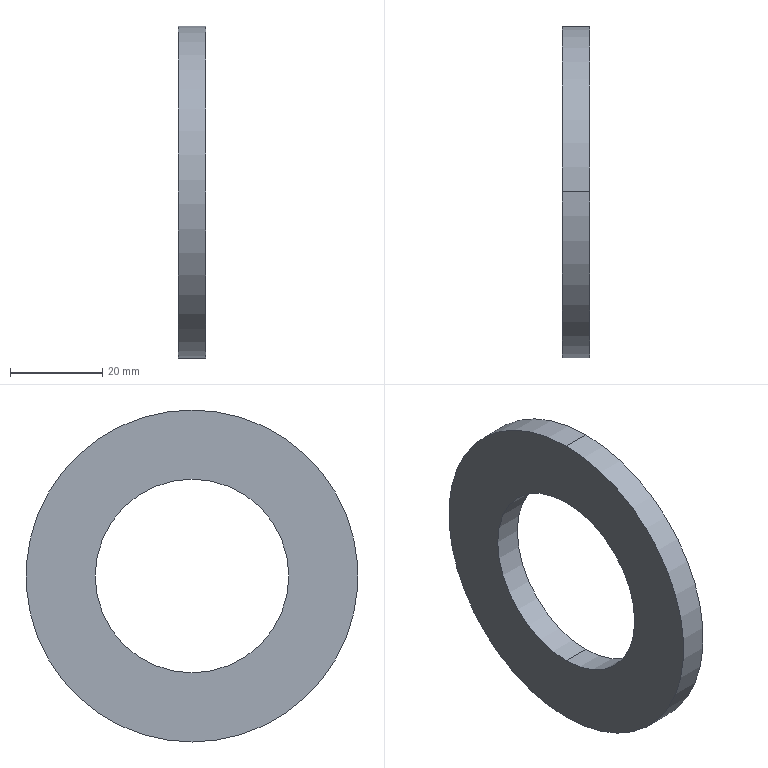Part | STEP file | 1 solid | 6 faces | box 6 x 72 x 72 mm | volume 16116 mm3 | cylinder 4 | plane 2 | commonest cylinder face diameters 42 x2 72 x2
STEP:
#1=CARTESIAN_POINT('',(0.,0.,0.));
#2=DIRECTION('',(0.,0.,1.));
#3=DIRECTION('',(1.,0.,0.));
#4=AXIS2_PLACEMENT_3D('',#1,#2,#3);
#5=CARTESIAN_POINT('',(0.,0.,36.));
#6=VERTEX_POINT('',#5);
#7=CARTESIAN_POINT('',(0.,0.,-36.));
#8=VERTEX_POINT('',#7);
#9=CARTESIAN_POINT('',(0.,0.,0.));
#10=DIRECTION('',(-1.,0.,0.));
#11=DIRECTION('',(0.,0.,-1.));
#12=AXIS2_PLACEMENT_3D('',#9,#10,#11);
#13=CIRCLE('',#12,36.);
#14=CARTESIAN_POINT('',(0.,0.,0.));
#15=DIRECTION('',(1.,0.,0.));
#16=DIRECTION('',(0.,0.,-1.));
#17=AXIS2_PLACEMENT_3D('',#14,#15,#16);
#18=CYLINDRICAL_SURFACE('',#17,36.);
#19=CARTESIAN_POINT('',(6.283,0.));
#20=DIRECTION('',(-1.,0.));
#21=VECTOR('',#20,1.);
#22=LINE('',#19,#21);
#23=(GEOMETRIC_REPRESENTATION_CONTEXT(2)PARAMETRIC_REPRESENTATION_CONTEXT()REPRESENTATION_CONTEXT('',''));
#24=DEFINITIONAL_REPRESENTATION('',(#22),#23);
#25=PCURVE('',#18,#24);
#26=CARTESIAN_POINT('',(0.,0.,0.));
#27=DIRECTION('',(-1.,0.,0.));
#28=DIRECTION('',(0.,0.,1.));
#29=AXIS2_PLACEMENT_3D('',#26,#27,#28);
#30=PLANE('',#29);
#31=CARTESIAN_POINT('',(0.,0.));
#32=DIRECTION('',(-1.,0.));
#33=AXIS2_PLACEMENT_2D('',#31,#32);
#34=CIRCLE('',#33,36.);
#35=(GEOMETRIC_REPRESENTATION_CONTEXT(2)PARAMETRIC_REPRESENTATION_CONTEXT()REPRESENTATION_CONTEXT('',''));
#36=DEFINITIONAL_REPRESENTATION('',(#34),#35);
#37=PCURVE('',#30,#36);
#38=SURFACE_CURVE('',#13,(#25,#37),.PCURVE_S1.);
#39=EDGE_CURVE('',#6,#8,#38,.T.);
#40=ORIENTED_EDGE('',*,*,#39,.F.);
#41=CARTESIAN_POINT('',(6.,0.,36.));
#42=VERTEX_POINT('',#41);
#43=CARTESIAN_POINT('',(0.,0.,36.));
#44=DIRECTION('',(1.,0.,0.));
#45=VECTOR('',#44,1.);
#46=LINE('',#43,#45);
#47=CARTESIAN_POINT('',(3.142,0.));
#48=DIRECTION('',(0.,1.));
#49=VECTOR('',#48,1.);
#50=LINE('',#47,#49);
#51=(GEOMETRIC_REPRESENTATION_CONTEXT(2)PARAMETRIC_REPRESENTATION_CONTEXT()REPRESENTATION_CONTEXT('',''));
#52=DEFINITIONAL_REPRESENTATION('',(#50),#51);
#53=PCURVE('',#18,#52);
#54=CARTESIAN_POINT('',(0.,0.,0.));
#55=DIRECTION('',(1.,0.,0.));
#56=DIRECTION('',(0.,0.,-1.));
#57=AXIS2_PLACEMENT_3D('',#54,#55,#56);
#58=CYLINDRICAL_SURFACE('',#57,36.);
#59=CARTESIAN_POINT('',(3.142,0.));
#60=DIRECTION('',(0.,1.));
#61=VECTOR('',#60,1.);
#62=LINE('',#59,#61);
#63=(GEOMETRIC_REPRESENTATION_CONTEXT(2)PARAMETRIC_REPRESENTATION_CONTEXT()REPRESENTATION_CONTEXT('',''));
#64=DEFINITIONAL_REPRESENTATION('',(#62),#63);
#65=PCURVE('',#58,#64);
#66=SURFACE_CURVE('',#46,(#53,#65),.PCURVE_S1.);
#67=EDGE_CURVE('',#6,#42,#66,.T.);
#68=ORIENTED_EDGE('',*,*,#67,.T.);
#69=CARTESIAN_POINT('',(6.,0.,-36.));
#70=VERTEX_POINT('',#69);
#71=CARTESIAN_POINT('',(6.,0.,0.));
#72=DIRECTION('',(-1.,0.,0.));
#73=DIRECTION('',(0.,0.,-1.));
#74=AXIS2_PLACEMENT_3D('',#71,#72,#73);
#75=CIRCLE('',#74,36.);
#76=CARTESIAN_POINT('',(6.283,6.));
#77=DIRECTION('',(-1.,0.));
#78=VECTOR('',#77,1.);
#79=LINE('',#76,#78);
#80=(GEOMETRIC_REPRESENTATION_CONTEXT(2)PARAMETRIC_REPRESENTATION_CONTEXT()REPRESENTATION_CONTEXT('',''));
#81=DEFINITIONAL_REPRESENTATION('',(#79),#80);
#82=PCURVE('',#18,#81);
#83=CARTESIAN_POINT('',(6.,0.,0.));
#84=DIRECTION('',(-1.,0.,0.));
#85=DIRECTION('',(0.,0.,1.));
#86=AXIS2_PLACEMENT_3D('',#83,#84,#85);
#87=PLANE('',#86);
#88=CARTESIAN_POINT('',(0.,0.));
#89=DIRECTION('',(-1.,0.));
#90=AXIS2_PLACEMENT_2D('',#88,#89);
#91=CIRCLE('',#90,36.);
#92=(GEOMETRIC_REPRESENTATION_CONTEXT(2)PARAMETRIC_REPRESENTATION_CONTEXT()REPRESENTATION_CONTEXT('',''));
#93=DEFINITIONAL_REPRESENTATION('',(#91),#92);
#94=PCURVE('',#87,#93);
#95=SURFACE_CURVE('',#75,(#82,#94),.PCURVE_S1.);
#96=EDGE_CURVE('',#42,#70,#95,.T.);
#97=ORIENTED_EDGE('',*,*,#96,.T.);
#98=CARTESIAN_POINT('',(0.,0.,-36.));
#99=DIRECTION('',(1.,0.,0.));
#100=VECTOR('',#99,1.);
#101=LINE('',#98,#100);
#102=CARTESIAN_POINT('',(0.,0.));
#103=DIRECTION('',(0.,1.));
#104=VECTOR('',#103,1.);
#105=LINE('',#102,#104);
#106=(GEOMETRIC_REPRESENTATION_CONTEXT(2)PARAMETRIC_REPRESENTATION_CONTEXT()REPRESENTATION_CONTEXT('',''));
#107=DEFINITIONAL_REPRESENTATION('',(#105),#106);
#108=PCURVE('',#18,#107);
#109=CARTESIAN_POINT('',(6.283,0.));
#110=DIRECTION('',(0.,1.));
#111=VECTOR('',#110,1.);
#112=LINE('',#109,#111);
#113=(GEOMETRIC_REPRESENTATION_CONTEXT(2)PARAMETRIC_REPRESENTATION_CONTEXT()REPRESENTATION_CONTEXT('',''));
#114=DEFINITIONAL_REPRESENTATION('',(#112),#113);
#115=PCURVE('',#58,#114);
#116=SURFACE_CURVE('',#101,(#108,#115),.PCURVE_S1.);
#117=EDGE_CURVE('',#8,#70,#116,.T.);
#118=ORIENTED_EDGE('',*,*,#117,.F.);
#119=EDGE_LOOP('',(#40,#68,#97,#118));
#120=FACE_BOUND('',#119,.T.);
#121=ADVANCED_FACE('',(#120),#18,.T.);
#122=CARTESIAN_POINT('',(0.,0.,-21.));
#123=VERTEX_POINT('',#122);
#124=CARTESIAN_POINT('',(6.,0.,-21.));
#125=VERTEX_POINT('',#124);
#126=CARTESIAN_POINT('',(0.,0.,-21.));
#127=DIRECTION('',(1.,0.,0.));
#128=VECTOR('',#127,1.);
#129=LINE('',#126,#128);
#130=CARTESIAN_POINT('',(0.,0.,0.));
#131=DIRECTION('',(1.,0.,0.));
#132=DIRECTION('',(0.,0.,-1.));
#133=AXIS2_PLACEMENT_3D('',#130,#131,#132);
#134=CYLINDRICAL_SURFACE('',#133,21.);
#135=CARTESIAN_POINT('',(6.283,0.));
#136=DIRECTION('',(0.,1.));
#137=VECTOR('',#136,1.);
#138=LINE('',#135,#137);
#139=(GEOMETRIC_REPRESENTATION_CONTEXT(2)PARAMETRIC_REPRESENTATION_CONTEXT()REPRESENTATION_CONTEXT('',''));
#140=DEFINITIONAL_REPRESENTATION('',(#138),#139);
#141=PCURVE('',#134,#140);
#142=CARTESIAN_POINT('',(0.,0.,0.));
#143=DIRECTION('',(1.,0.,0.));
#144=DIRECTION('',(0.,0.,-1.));
#145=AXIS2_PLACEMENT_3D('',#142,#143,#144);
#146=CYLINDRICAL_SURFACE('',#145,21.);
#147=CARTESIAN_POINT('',(0.,0.));
#148=DIRECTION('',(0.,1.));
#149=VECTOR('',#148,1.);
#150=LINE('',#147,#149);
#151=(GEOMETRIC_REPRESENTATION_CONTEXT(2)PARAMETRIC_REPRESENTATION_CONTEXT()REPRESENTATION_CONTEXT('',''));
#152=DEFINITIONAL_REPRESENTATION('',(#150),#151);
#153=PCURVE('',#146,#152);
#154=SURFACE_CURVE('',#129,(#141,#153),.PCURVE_S1.);
#155=EDGE_CURVE('',#123,#125,#154,.T.);
#156=ORIENTED_EDGE('',*,*,#155,.T.);
#157=CARTESIAN_POINT('',(6.,0.,21.));
#158=VERTEX_POINT('',#157);
#159=CARTESIAN_POINT('',(6.,0.,0.));
#160=DIRECTION('',(-1.,0.,0.));
#161=DIRECTION('',(0.,0.,-1.));
#162=AXIS2_PLACEMENT_3D('',#159,#160,#161);
#163=CIRCLE('',#162,21.);
#164=CARTESIAN_POINT('',(6.283,6.));
#165=DIRECTION('',(-1.,0.));
#166=VECTOR('',#165,1.);
#167=LINE('',#164,#166);
#168=(GEOMETRIC_REPRESENTATION_CONTEXT(2)PARAMETRIC_REPRESENTATION_CONTEXT()REPRESENTATION_CONTEXT('',''));
#169=DEFINITIONAL_REPRESENTATION('',(#167),#168);
#170=PCURVE('',#134,#169);
#171=CARTESIAN_POINT('',(0.,0.));
#172=DIRECTION('',(-1.,0.));
#173=AXIS2_PLACEMENT_2D('',#171,#172);
#174=CIRCLE('',#173,21.);
#175=(GEOMETRIC_REPRESENTATION_CONTEXT(2)PARAMETRIC_REPRESENTATION_CONTEXT()REPRESENTATION_CONTEXT('',''));
#176=DEFINITIONAL_REPRESENTATION('',(#174),#175);
#177=PCURVE('',#87,#176);
#178=SURFACE_CURVE('',#163,(#170,#177),.PCURVE_S1.);
#179=EDGE_CURVE('',#125,#158,#178,.T.);
#180=ORIENTED_EDGE('',*,*,#179,.T.);
#181=CARTESIAN_POINT('',(0.,0.,21.));
#182=VERTEX_POINT('',#181);
#183=CARTESIAN_POINT('',(0.,0.,21.));
#184=DIRECTION('',(1.,0.,0.));
#185=VECTOR('',#184,1.);
#186=LINE('',#183,#185);
#187=CARTESIAN_POINT('',(3.142,0.));
#188=DIRECTION('',(0.,1.));
#189=VECTOR('',#188,1.);
#190=LINE('',#187,#189);
#191=(GEOMETRIC_REPRESENTATION_CONTEXT(2)PARAMETRIC_REPRESENTATION_CONTEXT()REPRESENTATION_CONTEXT('',''));
#192=DEFINITIONAL_REPRESENTATION('',(#190),#191);
#193=PCURVE('',#134,#192);
#194=CARTESIAN_POINT('',(3.142,0.));
#195=DIRECTION('',(0.,1.));
#196=VECTOR('',#195,1.);
#197=LINE('',#194,#196);
#198=(GEOMETRIC_REPRESENTATION_CONTEXT(2)PARAMETRIC_REPRESENTATION_CONTEXT()REPRESENTATION_CONTEXT('',''));
#199=DEFINITIONAL_REPRESENTATION('',(#197),#198);
#200=PCURVE('',#146,#199);
#201=SURFACE_CURVE('',#186,(#193,#200),.PCURVE_S1.);
#202=EDGE_CURVE('',#182,#158,#201,.T.);
#203=ORIENTED_EDGE('',*,*,#202,.F.);
#204=CARTESIAN_POINT('',(0.,0.,0.));
#205=DIRECTION('',(1.,0.,0.));
#206=DIRECTION('',(0.,0.,-1.));
#207=AXIS2_PLACEMENT_3D('',#204,#205,#206);
#208=CIRCLE('',#207,21.);
#209=CARTESIAN_POINT('',(0.,0.));
#210=DIRECTION('',(1.,0.));
#211=VECTOR('',#210,1.);
#212=LINE('',#209,#211);
#213=(GEOMETRIC_REPRESENTATION_CONTEXT(2)PARAMETRIC_REPRESENTATION_CONTEXT()REPRESENTATION_CONTEXT('',''));
#214=DEFINITIONAL_REPRESENTATION('',(#212),#213);
#215=PCURVE('',#134,#214);
#216=CARTESIAN_POINT('',(-21.,0.));
#217=CARTESIAN_POINT('',(-21.,36.373));
#218=CARTESIAN_POINT('',(10.5,18.187));
#219=CARTESIAN_POINT('',(42.,0.));
#220=CARTESIAN_POINT('',(10.5,-18.187));
#221=CARTESIAN_POINT('',(-21.,-36.373));
#222=CARTESIAN_POINT('',(-21.,0.));
#223=(BOUNDED_CURVE()B_SPLINE_CURVE(2,(#216,#217,#218,#219,#220,#221,#222),.UNSPECIFIED.,.T.,.F.)B_SPLINE_CURVE_WITH_KNOTS((1,2,2,2,2,1),(-2.094,0.,2.094,4.189,6.283,8.378),.UNSPECIFIED.)CURVE()GEOMETRIC_REPRESENTATION_ITEM()RATIONAL_B_SPLINE_CURVE((1.,0.5,1.,0.5,1.,0.5,1.))REPRESENTATION_ITEM(''));
#224=(GEOMETRIC_REPRESENTATION_CONTEXT(2)PARAMETRIC_REPRESENTATION_CONTEXT()REPRESENTATION_CONTEXT('',''));
#225=DEFINITIONAL_REPRESENTATION('',(#223),#224);
#226=PCURVE('',#30,#225);
#227=SURFACE_CURVE('',#208,(#215,#226),.PCURVE_S1.);
#228=EDGE_CURVE('',#182,#123,#227,.T.);
#229=ORIENTED_EDGE('',*,*,#228,.T.);
#230=EDGE_LOOP('',(#156,#180,#203,#229));
#231=FACE_BOUND('',#230,.F.);
#232=ADVANCED_FACE('',(#231),#134,.F.);
#233=CARTESIAN_POINT('',(0.,0.,0.));
#234=DIRECTION('',(-1.,0.,0.));
#235=DIRECTION('',(0.,0.,-1.));
#236=AXIS2_PLACEMENT_3D('',#233,#234,#235);
#237=CIRCLE('',#236,36.);
#238=CARTESIAN_POINT('',(0.,0.));
#239=DIRECTION('',(-1.,0.));
#240=AXIS2_PLACEMENT_2D('',#238,#239);
#241=CIRCLE('',#240,36.);
#242=(GEOMETRIC_REPRESENTATION_CONTEXT(2)PARAMETRIC_REPRESENTATION_CONTEXT()REPRESENTATION_CONTEXT('',''));
#243=DEFINITIONAL_REPRESENTATION('',(#241),#242);
#244=PCURVE('',#30,#243);
#245=CARTESIAN_POINT('',(6.283,0.));
#246=DIRECTION('',(-1.,0.));
#247=VECTOR('',#246,1.);
#248=LINE('',#245,#247);
#249=(GEOMETRIC_REPRESENTATION_CONTEXT(2)PARAMETRIC_REPRESENTATION_CONTEXT()REPRESENTATION_CONTEXT('',''));
#250=DEFINITIONAL_REPRESENTATION('',(#248),#249);
#251=PCURVE('',#58,#250);
#252=SURFACE_CURVE('',#237,(#244,#251),.PCURVE_S1.);
#253=EDGE_CURVE('',#8,#6,#252,.T.);
#254=ORIENTED_EDGE('',*,*,#253,.T.);
#255=ORIENTED_EDGE('',*,*,#39,.T.);
#256=EDGE_LOOP('',(#254,#255));
#257=FACE_BOUND('',#256,.T.);
#258=CARTESIAN_POINT('',(0.,0.,0.));
#259=DIRECTION('',(1.,0.,0.));
#260=DIRECTION('',(0.,0.,-1.));
#261=AXIS2_PLACEMENT_3D('',#258,#259,#260);
#262=CIRCLE('',#261,21.);
#263=CARTESIAN_POINT('',(-21.,0.));
#264=CARTESIAN_POINT('',(-21.,36.373));
#265=CARTESIAN_POINT('',(10.5,18.187));
#266=CARTESIAN_POINT('',(42.,0.));
#267=CARTESIAN_POINT('',(10.5,-18.187));
#268=CARTESIAN_POINT('',(-21.,-36.373));
#269=CARTESIAN_POINT('',(-21.,0.));
#270=(BOUNDED_CURVE()B_SPLINE_CURVE(2,(#263,#264,#265,#266,#267,#268,#269),.UNSPECIFIED.,.T.,.F.)B_SPLINE_CURVE_WITH_KNOTS((1,2,2,2,2,1),(-2.094,0.,2.094,4.189,6.283,8.378),.UNSPECIFIED.)CURVE()GEOMETRIC_REPRESENTATION_ITEM()RATIONAL_B_SPLINE_CURVE((1.,0.5,1.,0.5,1.,0.5,1.))REPRESENTATION_ITEM(''));
#271=(GEOMETRIC_REPRESENTATION_CONTEXT(2)PARAMETRIC_REPRESENTATION_CONTEXT()REPRESENTATION_CONTEXT('',''));
#272=DEFINITIONAL_REPRESENTATION('',(#270),#271);
#273=PCURVE('',#30,#272);
#274=CARTESIAN_POINT('',(0.,0.));
#275=DIRECTION('',(1.,0.));
#276=VECTOR('',#275,1.);
#277=LINE('',#274,#276);
#278=(GEOMETRIC_REPRESENTATION_CONTEXT(2)PARAMETRIC_REPRESENTATION_CONTEXT()REPRESENTATION_CONTEXT('',''));
#279=DEFINITIONAL_REPRESENTATION('',(#277),#278);
#280=PCURVE('',#146,#279);
#281=SURFACE_CURVE('',#262,(#273,#280),.PCURVE_S1.);
#282=EDGE_CURVE('',#123,#182,#281,.T.);
#283=ORIENTED_EDGE('',*,*,#282,.T.);
#284=ORIENTED_EDGE('',*,*,#228,.T.);
#285=EDGE_LOOP('',(#283,#284));
#286=FACE_BOUND('',#285,.T.);
#287=ADVANCED_FACE('',(#257,#286),#30,.T.);
#288=ORIENTED_EDGE('',*,*,#67,.F.);
#289=ORIENTED_EDGE('',*,*,#253,.F.);
#290=ORIENTED_EDGE('',*,*,#117,.T.);
#291=CARTESIAN_POINT('',(6.,0.,0.));
#292=DIRECTION('',(-1.,0.,0.));
#293=DIRECTION('',(0.,0.,-1.));
#294=AXIS2_PLACEMENT_3D('',#291,#292,#293);
#295=CIRCLE('',#294,36.);
#296=CARTESIAN_POINT('',(6.283,6.));
#297=DIRECTION('',(-1.,0.));
#298=VECTOR('',#297,1.);
#299=LINE('',#296,#298);
#300=(GEOMETRIC_REPRESENTATION_CONTEXT(2)PARAMETRIC_REPRESENTATION_CONTEXT()REPRESENTATION_CONTEXT('',''));
#301=DEFINITIONAL_REPRESENTATION('',(#299),#300);
#302=PCURVE('',#58,#301);
#303=CARTESIAN_POINT('',(0.,0.));
#304=DIRECTION('',(-1.,0.));
#305=AXIS2_PLACEMENT_2D('',#303,#304);
#306=CIRCLE('',#305,36.);
#307=(GEOMETRIC_REPRESENTATION_CONTEXT(2)PARAMETRIC_REPRESENTATION_CONTEXT()REPRESENTATION_CONTEXT('',''));
#308=DEFINITIONAL_REPRESENTATION('',(#306),#307);
#309=PCURVE('',#87,#308);
#310=SURFACE_CURVE('',#295,(#302,#309),.PCURVE_S1.);
#311=EDGE_CURVE('',#70,#42,#310,.T.);
#312=ORIENTED_EDGE('',*,*,#311,.T.);
#313=EDGE_LOOP('',(#288,#289,#290,#312));
#314=FACE_BOUND('',#313,.T.);
#315=ADVANCED_FACE('',(#314),#58,.T.);
#316=CARTESIAN_POINT('',(6.,0.,0.));
#317=DIRECTION('',(-1.,0.,0.));
#318=DIRECTION('',(0.,0.,-1.));
#319=AXIS2_PLACEMENT_3D('',#316,#317,#318);
#320=CIRCLE('',#319,21.);
#321=CARTESIAN_POINT('',(6.283,6.));
#322=DIRECTION('',(-1.,0.));
#323=VECTOR('',#322,1.);
#324=LINE('',#321,#323);
#325=(GEOMETRIC_REPRESENTATION_CONTEXT(2)PARAMETRIC_REPRESENTATION_CONTEXT()REPRESENTATION_CONTEXT('',''));
#326=DEFINITIONAL_REPRESENTATION('',(#324),#325);
#327=PCURVE('',#146,#326);
#328=CARTESIAN_POINT('',(0.,0.));
#329=DIRECTION('',(-1.,0.));
#330=AXIS2_PLACEMENT_2D('',#328,#329);
#331=CIRCLE('',#330,21.);
#332=(GEOMETRIC_REPRESENTATION_CONTEXT(2)PARAMETRIC_REPRESENTATION_CONTEXT()REPRESENTATION_CONTEXT('',''));
#333=DEFINITIONAL_REPRESENTATION('',(#331),#332);
#334=PCURVE('',#87,#333);
#335=SURFACE_CURVE('',#320,(#327,#334),.PCURVE_S1.);
#336=EDGE_CURVE('',#158,#125,#335,.T.);
#337=ORIENTED_EDGE('',*,*,#336,.T.);
#338=ORIENTED_EDGE('',*,*,#155,.F.);
#339=ORIENTED_EDGE('',*,*,#282,.T.);
#340=ORIENTED_EDGE('',*,*,#202,.T.);
#341=EDGE_LOOP('',(#337,#338,#339,#340));
#342=FACE_BOUND('',#341,.F.);
#343=ADVANCED_FACE('',(#342),#146,.F.);
#344=ORIENTED_EDGE('',*,*,#311,.F.);
#345=ORIENTED_EDGE('',*,*,#96,.F.);
#346=EDGE_LOOP('',(#344,#345));
#347=FACE_BOUND('',#346,.T.);
#348=ORIENTED_EDGE('',*,*,#179,.T.);
#349=ORIENTED_EDGE('',*,*,#336,.T.);
#350=EDGE_LOOP('',(#348,#349));
#351=FACE_BOUND('',#350,.T.);
#352=ADVANCED_FACE('',(#347,#351),#87,.F.);
#353=CLOSED_SHELL('',(#121,#232,#287,#315,#343,#352));
#354=MANIFOLD_SOLID_BREP('',#353);
#355=(LENGTH_UNIT()NAMED_UNIT(*)SI_UNIT(.MILLI.,.METRE.));
#356=UNCERTAINTY_MEASURE_WITH_UNIT(LENGTH_MEASURE(0.0000001),#355,'','');
#357=(NAMED_UNIT(*)PLANE_ANGLE_UNIT()SI_UNIT($,.RADIAN.));
#358=(NAMED_UNIT(*)SI_UNIT($,.STERADIAN.)SOLID_ANGLE_UNIT());
#359=(GEOMETRIC_REPRESENTATION_CONTEXT(3)GLOBAL_UNCERTAINTY_ASSIGNED_CONTEXT((#356))GLOBAL_UNIT_ASSIGNED_CONTEXT((#355,#357,#358))REPRESENTATION_CONTEXT('',''));
#360=ADVANCED_BREP_SHAPE_REPRESENTATION('',(#4,#354),#359);